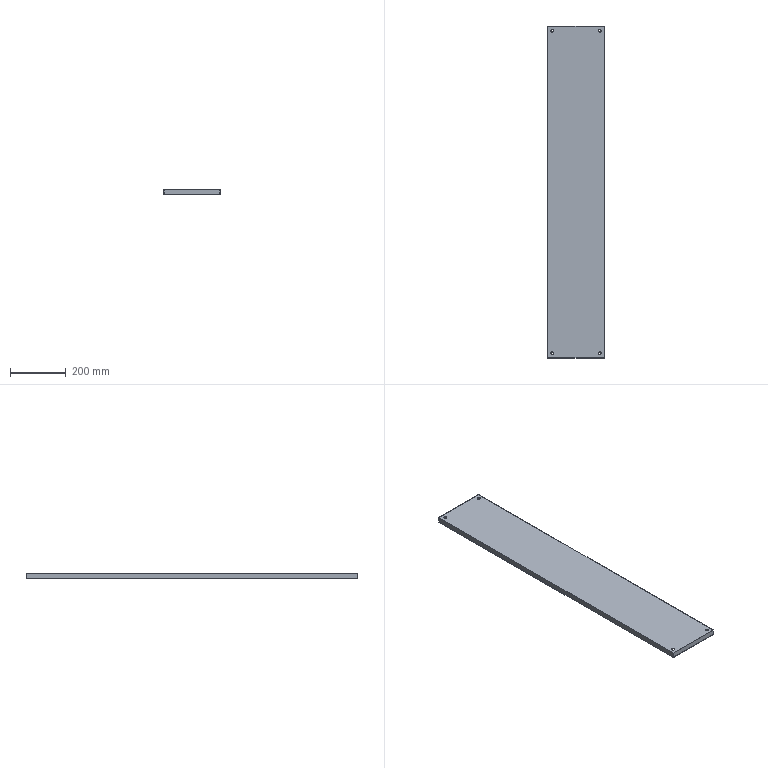Part | SolidWorks | features Extrusion 1, HoleWzd 1, ICE 1, Shell 1 | 1 solid | 32 faces | box 204 x 1196 x 20 mm | volume 684802 mm3 | cylinder 16 | plane 16 | commonest cylinder face diameters 6.6 x8 11 x8
STEP:
#1=CARTESIAN_POINT('',(-79.5,580.75,18.));
#2=VERTEX_POINT('',#1);
#3=CARTESIAN_POINT('',(-90.5,580.75,18.));
#4=VERTEX_POINT('',#3);
#5=CARTESIAN_POINT('',(-85.,580.75,18.));
#6=DIRECTION('',(0.,0.,-1.));
#7=DIRECTION('',(-1.,0.,0.));
#8=AXIS2_PLACEMENT_3D('',#5,#6,#7);
#9=CIRCLE('',#8,5.5);
#10=EDGE_CURVE('',#2,#4,#9,.T.);
#11=ORIENTED_EDGE('',*,*,#10,.T.);
#12=CARTESIAN_POINT('',(-90.5,580.75,20.));
#13=VERTEX_POINT('',#12);
#14=CARTESIAN_POINT('',(-90.5,580.75,20.));
#15=DIRECTION('',(0.,0.,1.));
#16=VECTOR('',#15,1000.);
#17=LINE('',#14,#16);
#18=EDGE_CURVE('',#4,#13,#17,.T.);
#19=ORIENTED_EDGE('',*,*,#18,.T.);
#20=CARTESIAN_POINT('',(-79.5,580.75,20.));
#21=VERTEX_POINT('',#20);
#22=CARTESIAN_POINT('',(-85.,580.75,20.));
#23=DIRECTION('',(0.,0.,1.));
#24=DIRECTION('',(1.,0.,0.));
#25=AXIS2_PLACEMENT_3D('',#22,#23,#24);
#26=CIRCLE('',#25,5.5);
#27=EDGE_CURVE('',#13,#21,#26,.T.);
#28=ORIENTED_EDGE('',*,*,#27,.T.);
#29=CARTESIAN_POINT('',(-79.5,580.75,20.));
#30=DIRECTION('',(0.,0.,1.));
#31=VECTOR('',#30,1000.);
#32=LINE('',#29,#31);
#33=EDGE_CURVE('',#2,#21,#32,.T.);
#34=ORIENTED_EDGE('',*,*,#33,.F.);
#35=EDGE_LOOP('',(#11,#19,#28,#34));
#36=FACE_OUTER_BOUND('',#35,.T.);
#37=CARTESIAN_POINT('',(-85.,580.75,20.));
#38=DIRECTION('',(0.,0.,1.));
#39=DIRECTION('',(1.,0.,0.));
#40=AXIS2_PLACEMENT_3D('',#37,#38,#39);
#41=CYLINDRICAL_SURFACE('',#40,5.5);
#42=ADVANCED_FACE('',(#36),#41,.F.);
#43=CARTESIAN_POINT('',(-88.3,580.75,0.));
#44=VERTEX_POINT('',#43);
#45=CARTESIAN_POINT('',(-81.7,580.75,0.));
#46=VERTEX_POINT('',#45);
#47=CARTESIAN_POINT('',(-85.,580.75,0.));
#48=DIRECTION('',(0.,0.,1.));
#49=DIRECTION('',(1.,0.,0.));
#50=AXIS2_PLACEMENT_3D('',#47,#48,#49);
#51=CIRCLE('',#50,3.3);
#52=EDGE_CURVE('',#44,#46,#51,.T.);
#53=ORIENTED_EDGE('',*,*,#52,.F.);
#54=CARTESIAN_POINT('',(-88.3,580.75,2.));
#55=VERTEX_POINT('',#54);
#56=CARTESIAN_POINT('',(-88.3,580.75,20.));
#57=DIRECTION('',(0.,0.,1.));
#58=VECTOR('',#57,1000.);
#59=LINE('',#56,#58);
#60=EDGE_CURVE('',#44,#55,#59,.T.);
#61=ORIENTED_EDGE('',*,*,#60,.T.);
#62=CARTESIAN_POINT('',(-81.7,580.75,2.));
#63=VERTEX_POINT('',#62);
#64=CARTESIAN_POINT('',(-85.,580.75,2.));
#65=DIRECTION('',(0.,0.,-1.));
#66=DIRECTION('',(-1.,0.,0.));
#67=AXIS2_PLACEMENT_3D('',#64,#65,#66);
#68=CIRCLE('',#67,3.3);
#69=EDGE_CURVE('',#63,#55,#68,.T.);
#70=ORIENTED_EDGE('',*,*,#69,.F.);
#71=CARTESIAN_POINT('',(-81.7,580.75,20.));
#72=DIRECTION('',(0.,0.,1.));
#73=VECTOR('',#72,1000.);
#74=LINE('',#71,#73);
#75=EDGE_CURVE('',#46,#63,#74,.T.);
#76=ORIENTED_EDGE('',*,*,#75,.F.);
#77=EDGE_LOOP('',(#53,#61,#70,#76));
#78=FACE_OUTER_BOUND('',#77,.T.);
#79=CARTESIAN_POINT('',(-85.,580.75,20.));
#80=DIRECTION('',(0.,0.,1.));
#81=DIRECTION('',(1.,0.,0.));
#82=AXIS2_PLACEMENT_3D('',#79,#80,#81);
#83=CYLINDRICAL_SURFACE('',#82,3.3);
#84=ADVANCED_FACE('',(#78),#83,.F.);
#85=CARTESIAN_POINT('',(-88.3,-580.75,0.));
#86=VERTEX_POINT('',#85);
#87=CARTESIAN_POINT('',(-81.7,-580.75,0.));
#88=VERTEX_POINT('',#87);
#89=CARTESIAN_POINT('',(-85.,-580.75,0.));
#90=DIRECTION('',(0.,0.,1.));
#91=DIRECTION('',(1.,0.,0.));
#92=AXIS2_PLACEMENT_3D('',#89,#90,#91);
#93=CIRCLE('',#92,3.3);
#94=EDGE_CURVE('',#86,#88,#93,.T.);
#95=ORIENTED_EDGE('',*,*,#94,.F.);
#96=CARTESIAN_POINT('',(-88.3,-580.75,2.));
#97=VERTEX_POINT('',#96);
#98=CARTESIAN_POINT('',(-88.3,-580.75,20.));
#99=DIRECTION('',(0.,0.,1.));
#100=VECTOR('',#99,1000.);
#101=LINE('',#98,#100);
#102=EDGE_CURVE('',#86,#97,#101,.T.);
#103=ORIENTED_EDGE('',*,*,#102,.T.);
#104=CARTESIAN_POINT('',(-81.7,-580.75,2.));
#105=VERTEX_POINT('',#104);
#106=CARTESIAN_POINT('',(-85.,-580.75,2.));
#107=DIRECTION('',(0.,0.,-1.));
#108=DIRECTION('',(-1.,0.,0.));
#109=AXIS2_PLACEMENT_3D('',#106,#107,#108);
#110=CIRCLE('',#109,3.3);
#111=EDGE_CURVE('',#105,#97,#110,.T.);
#112=ORIENTED_EDGE('',*,*,#111,.F.);
#113=CARTESIAN_POINT('',(-81.7,-580.75,20.));
#114=DIRECTION('',(0.,0.,1.));
#115=VECTOR('',#114,1000.);
#116=LINE('',#113,#115);
#117=EDGE_CURVE('',#88,#105,#116,.T.);
#118=ORIENTED_EDGE('',*,*,#117,.F.);
#119=EDGE_LOOP('',(#95,#103,#112,#118));
#120=FACE_OUTER_BOUND('',#119,.T.);
#121=CARTESIAN_POINT('',(-85.,-580.75,20.));
#122=DIRECTION('',(0.,0.,1.));
#123=DIRECTION('',(1.,0.,0.));
#124=AXIS2_PLACEMENT_3D('',#121,#122,#123);
#125=CYLINDRICAL_SURFACE('',#124,3.3);
#126=ADVANCED_FACE('',(#120),#125,.F.);
#127=CARTESIAN_POINT('',(-79.5,-580.75,18.));
#128=VERTEX_POINT('',#127);
#129=CARTESIAN_POINT('',(-90.5,-580.75,18.));
#130=VERTEX_POINT('',#129);
#131=CARTESIAN_POINT('',(-85.,-580.75,18.));
#132=DIRECTION('',(0.,0.,-1.));
#133=DIRECTION('',(-1.,0.,0.));
#134=AXIS2_PLACEMENT_3D('',#131,#132,#133);
#135=CIRCLE('',#134,5.5);
#136=EDGE_CURVE('',#128,#130,#135,.T.);
#137=ORIENTED_EDGE('',*,*,#136,.T.);
#138=CARTESIAN_POINT('',(-90.5,-580.75,20.));
#139=VERTEX_POINT('',#138);
#140=CARTESIAN_POINT('',(-90.5,-580.75,20.));
#141=DIRECTION('',(0.,0.,1.));
#142=VECTOR('',#141,1000.);
#143=LINE('',#140,#142);
#144=EDGE_CURVE('',#130,#139,#143,.T.);
#145=ORIENTED_EDGE('',*,*,#144,.T.);
#146=CARTESIAN_POINT('',(-79.5,-580.75,20.));
#147=VERTEX_POINT('',#146);
#148=CARTESIAN_POINT('',(-85.,-580.75,20.));
#149=DIRECTION('',(0.,0.,1.));
#150=DIRECTION('',(1.,0.,0.));
#151=AXIS2_PLACEMENT_3D('',#148,#149,#150);
#152=CIRCLE('',#151,5.5);
#153=EDGE_CURVE('',#139,#147,#152,.T.);
#154=ORIENTED_EDGE('',*,*,#153,.T.);
#155=CARTESIAN_POINT('',(-79.5,-580.75,20.));
#156=DIRECTION('',(0.,0.,1.));
#157=VECTOR('',#156,1000.);
#158=LINE('',#155,#157);
#159=EDGE_CURVE('',#128,#147,#158,.T.);
#160=ORIENTED_EDGE('',*,*,#159,.F.);
#161=EDGE_LOOP('',(#137,#145,#154,#160));
#162=FACE_OUTER_BOUND('',#161,.T.);
#163=CARTESIAN_POINT('',(-85.,-580.75,20.));
#164=DIRECTION('',(0.,0.,1.));
#165=DIRECTION('',(1.,0.,0.));
#166=AXIS2_PLACEMENT_3D('',#163,#164,#165);
#167=CYLINDRICAL_SURFACE('',#166,5.5);
#168=ADVANCED_FACE('',(#162),#167,.F.);
#169=CARTESIAN_POINT('',(90.5,-580.75,18.));
#170=VERTEX_POINT('',#169);
#171=CARTESIAN_POINT('',(79.5,-580.75,18.));
#172=VERTEX_POINT('',#171);
#173=CARTESIAN_POINT('',(85.,-580.75,18.));
#174=DIRECTION('',(0.,0.,-1.));
#175=DIRECTION('',(-1.,0.,0.));
#176=AXIS2_PLACEMENT_3D('',#173,#174,#175);
#177=CIRCLE('',#176,5.5);
#178=EDGE_CURVE('',#170,#172,#177,.T.);
#179=ORIENTED_EDGE('',*,*,#178,.T.);
#180=CARTESIAN_POINT('',(79.5,-580.75,20.));
#181=VERTEX_POINT('',#180);
#182=CARTESIAN_POINT('',(79.5,-580.75,20.));
#183=DIRECTION('',(0.,0.,1.));
#184=VECTOR('',#183,1000.);
#185=LINE('',#182,#184);
#186=EDGE_CURVE('',#172,#181,#185,.T.);
#187=ORIENTED_EDGE('',*,*,#186,.T.);
#188=CARTESIAN_POINT('',(90.5,-580.75,20.));
#189=VERTEX_POINT('',#188);
#190=CARTESIAN_POINT('',(85.,-580.75,20.));
#191=DIRECTION('',(0.,0.,1.));
#192=DIRECTION('',(1.,0.,0.));
#193=AXIS2_PLACEMENT_3D('',#190,#191,#192);
#194=CIRCLE('',#193,5.5);
#195=EDGE_CURVE('',#181,#189,#194,.T.);
#196=ORIENTED_EDGE('',*,*,#195,.T.);
#197=CARTESIAN_POINT('',(90.5,-580.75,20.));
#198=DIRECTION('',(0.,0.,1.));
#199=VECTOR('',#198,1000.);
#200=LINE('',#197,#199);
#201=EDGE_CURVE('',#170,#189,#200,.T.);
#202=ORIENTED_EDGE('',*,*,#201,.F.);
#203=EDGE_LOOP('',(#179,#187,#196,#202));
#204=FACE_OUTER_BOUND('',#203,.T.);
#205=CARTESIAN_POINT('',(85.,-580.75,20.));
#206=DIRECTION('',(0.,0.,1.));
#207=DIRECTION('',(1.,0.,0.));
#208=AXIS2_PLACEMENT_3D('',#205,#206,#207);
#209=CYLINDRICAL_SURFACE('',#208,5.5);
#210=ADVANCED_FACE('',(#204),#209,.F.);
#211=CARTESIAN_POINT('',(81.7,-580.75,0.));
#212=VERTEX_POINT('',#211);
#213=CARTESIAN_POINT('',(88.3,-580.75,0.));
#214=VERTEX_POINT('',#213);
#215=CARTESIAN_POINT('',(85.,-580.75,0.));
#216=DIRECTION('',(0.,0.,1.));
#217=DIRECTION('',(1.,0.,0.));
#218=AXIS2_PLACEMENT_3D('',#215,#216,#217);
#219=CIRCLE('',#218,3.3);
#220=EDGE_CURVE('',#212,#214,#219,.T.);
#221=ORIENTED_EDGE('',*,*,#220,.F.);
#222=CARTESIAN_POINT('',(81.7,-580.75,2.));
#223=VERTEX_POINT('',#222);
#224=CARTESIAN_POINT('',(81.7,-580.75,20.));
#225=DIRECTION('',(0.,0.,1.));
#226=VECTOR('',#225,1000.);
#227=LINE('',#224,#226);
#228=EDGE_CURVE('',#212,#223,#227,.T.);
#229=ORIENTED_EDGE('',*,*,#228,.T.);
#230=CARTESIAN_POINT('',(88.3,-580.75,2.));
#231=VERTEX_POINT('',#230);
#232=CARTESIAN_POINT('',(85.,-580.75,2.));
#233=DIRECTION('',(0.,0.,-1.));
#234=DIRECTION('',(-1.,0.,0.));
#235=AXIS2_PLACEMENT_3D('',#232,#233,#234);
#236=CIRCLE('',#235,3.3);
#237=EDGE_CURVE('',#231,#223,#236,.T.);
#238=ORIENTED_EDGE('',*,*,#237,.F.);
#239=CARTESIAN_POINT('',(88.3,-580.75,20.));
#240=DIRECTION('',(0.,0.,1.));
#241=VECTOR('',#240,1000.);
#242=LINE('',#239,#241);
#243=EDGE_CURVE('',#214,#231,#242,.T.);
#244=ORIENTED_EDGE('',*,*,#243,.F.);
#245=EDGE_LOOP('',(#221,#229,#238,#244));
#246=FACE_OUTER_BOUND('',#245,.T.);
#247=CARTESIAN_POINT('',(85.,-580.75,20.));
#248=DIRECTION('',(0.,0.,1.));
#249=DIRECTION('',(1.,0.,0.));
#250=AXIS2_PLACEMENT_3D('',#247,#248,#249);
#251=CYLINDRICAL_SURFACE('',#250,3.3);
#252=ADVANCED_FACE('',(#246),#251,.F.);
#253=CARTESIAN_POINT('',(81.7,580.75,0.));
#254=VERTEX_POINT('',#253);
#255=CARTESIAN_POINT('',(88.3,580.75,0.));
#256=VERTEX_POINT('',#255);
#257=CARTESIAN_POINT('',(85.,580.75,0.));
#258=DIRECTION('',(0.,0.,1.));
#259=DIRECTION('',(1.,0.,0.));
#260=AXIS2_PLACEMENT_3D('',#257,#258,#259);
#261=CIRCLE('',#260,3.3);
#262=EDGE_CURVE('',#254,#256,#261,.T.);
#263=ORIENTED_EDGE('',*,*,#262,.F.);
#264=CARTESIAN_POINT('',(81.7,580.75,2.));
#265=VERTEX_POINT('',#264);
#266=CARTESIAN_POINT('',(81.7,580.75,20.));
#267=DIRECTION('',(0.,0.,1.));
#268=VECTOR('',#267,1000.);
#269=LINE('',#266,#268);
#270=EDGE_CURVE('',#254,#265,#269,.T.);
#271=ORIENTED_EDGE('',*,*,#270,.T.);
#272=CARTESIAN_POINT('',(88.3,580.75,2.));
#273=VERTEX_POINT('',#272);
#274=CARTESIAN_POINT('',(85.,580.75,2.));
#275=DIRECTION('',(0.,0.,-1.));
#276=DIRECTION('',(-1.,0.,0.));
#277=AXIS2_PLACEMENT_3D('',#274,#275,#276);
#278=CIRCLE('',#277,3.3);
#279=EDGE_CURVE('',#273,#265,#278,.T.);
#280=ORIENTED_EDGE('',*,*,#279,.F.);
#281=CARTESIAN_POINT('',(88.3,580.75,20.));
#282=DIRECTION('',(0.,0.,1.));
#283=VECTOR('',#282,1000.);
#284=LINE('',#281,#283);
#285=EDGE_CURVE('',#256,#273,#284,.T.);
#286=ORIENTED_EDGE('',*,*,#285,.F.);
#287=EDGE_LOOP('',(#263,#271,#280,#286));
#288=FACE_OUTER_BOUND('',#287,.T.);
#289=CARTESIAN_POINT('',(85.,580.75,20.));
#290=DIRECTION('',(0.,0.,1.));
#291=DIRECTION('',(1.,0.,0.));
#292=AXIS2_PLACEMENT_3D('',#289,#290,#291);
#293=CYLINDRICAL_SURFACE('',#292,3.3);
#294=ADVANCED_FACE('',(#288),#293,.F.);
#295=CARTESIAN_POINT('',(90.5,580.75,18.));
#296=VERTEX_POINT('',#295);
#297=CARTESIAN_POINT('',(79.5,580.75,18.));
#298=VERTEX_POINT('',#297);
#299=CARTESIAN_POINT('',(85.,580.75,18.));
#300=DIRECTION('',(0.,0.,-1.));
#301=DIRECTION('',(-1.,0.,0.));
#302=AXIS2_PLACEMENT_3D('',#299,#300,#301);
#303=CIRCLE('',#302,5.5);
#304=EDGE_CURVE('',#296,#298,#303,.T.);
#305=ORIENTED_EDGE('',*,*,#304,.T.);
#306=CARTESIAN_POINT('',(79.5,580.75,20.));
#307=VERTEX_POINT('',#306);
#308=CARTESIAN_POINT('',(79.5,580.75,20.));
#309=DIRECTION('',(0.,0.,1.));
#310=VECTOR('',#309,1000.);
#311=LINE('',#308,#310);
#312=EDGE_CURVE('',#298,#307,#311,.T.);
#313=ORIENTED_EDGE('',*,*,#312,.T.);
#314=CARTESIAN_POINT('',(90.5,580.75,20.));
#315=VERTEX_POINT('',#314);
#316=CARTESIAN_POINT('',(85.,580.75,20.));
#317=DIRECTION('',(0.,0.,1.));
#318=DIRECTION('',(1.,0.,0.));
#319=AXIS2_PLACEMENT_3D('',#316,#317,#318);
#320=CIRCLE('',#319,5.5);
#321=EDGE_CURVE('',#307,#315,#320,.T.);
#322=ORIENTED_EDGE('',*,*,#321,.T.);
#323=CARTESIAN_POINT('',(90.5,580.75,20.));
#324=DIRECTION('',(0.,0.,1.));
#325=VECTOR('',#324,1000.);
#326=LINE('',#323,#325);
#327=EDGE_CURVE('',#296,#315,#326,.T.);
#328=ORIENTED_EDGE('',*,*,#327,.F.);
#329=EDGE_LOOP('',(#305,#313,#322,#328));
#330=FACE_OUTER_BOUND('',#329,.T.);
#331=CARTESIAN_POINT('',(85.,580.75,20.));
#332=DIRECTION('',(0.,0.,1.));
#333=DIRECTION('',(1.,0.,0.));
#334=AXIS2_PLACEMENT_3D('',#331,#332,#333);
#335=CYLINDRICAL_SURFACE('',#334,5.5);
#336=ADVANCED_FACE('',(#330),#335,.F.);
#337=CARTESIAN_POINT('',(85.,580.75,0.));
#338=DIRECTION('',(0.,0.,1.));
#339=DIRECTION('',(1.,0.,0.));
#340=AXIS2_PLACEMENT_3D('',#337,#338,#339);
#341=CIRCLE('',#340,3.3);
#342=EDGE_CURVE('',#256,#254,#341,.T.);
#343=ORIENTED_EDGE('',*,*,#342,.T.);
#344=ORIENTED_EDGE('',*,*,#262,.T.);
#345=EDGE_LOOP('',(#343,#344));
#346=FACE_BOUND('',#345,.T.);
#347=CARTESIAN_POINT('',(102.,-597.75,0.));
#348=VERTEX_POINT('',#347);
#349=CARTESIAN_POINT('',(102.,597.75,0.));
#350=VERTEX_POINT('',#349);
#351=CARTESIAN_POINT('',(102.,-597.75,0.));
#352=DIRECTION('',(0.,1.,0.));
#353=VECTOR('',#352,1000.);
#354=LINE('',#351,#353);
#355=EDGE_CURVE('',#348,#350,#354,.T.);
#356=ORIENTED_EDGE('',*,*,#355,.F.);
#357=CARTESIAN_POINT('',(-102.,-597.75,0.));
#358=VERTEX_POINT('',#357);
#359=CARTESIAN_POINT('',(-102.,-597.75,0.));
#360=DIRECTION('',(1.,0.,0.));
#361=VECTOR('',#360,1000.);
#362=LINE('',#359,#361);
#363=EDGE_CURVE('',#358,#348,#362,.T.);
#364=ORIENTED_EDGE('',*,*,#363,.F.);
#365=CARTESIAN_POINT('',(-102.,597.75,0.));
#366=VERTEX_POINT('',#365);
#367=CARTESIAN_POINT('',(-102.,-597.75,0.));
#368=DIRECTION('',(0.,-1.,0.));
#369=VECTOR('',#368,1000.);
#370=LINE('',#367,#369);
#371=EDGE_CURVE('',#366,#358,#370,.T.);
#372=ORIENTED_EDGE('',*,*,#371,.F.);
#373=CARTESIAN_POINT('',(-102.,597.75,0.));
#374=DIRECTION('',(-1.,0.,0.));
#375=VECTOR('',#374,1000.);
#376=LINE('',#373,#375);
#377=EDGE_CURVE('',#350,#366,#376,.T.);
#378=ORIENTED_EDGE('',*,*,#377,.F.);
#379=EDGE_LOOP('',(#356,#364,#372,#378));
#380=FACE_OUTER_BOUND('',#379,.T.);
#381=CARTESIAN_POINT('',(82.,-577.75,0.));
#382=VERTEX_POINT('',#381);
#383=CARTESIAN_POINT('',(-82.,-577.75,0.));
#384=VERTEX_POINT('',#383);
#385=CARTESIAN_POINT('',(82.,-577.75,0.));
#386=DIRECTION('',(-1.,0.,0.));
#387=VECTOR('',#386,1000.);
#388=LINE('',#385,#387);
#389=EDGE_CURVE('',#382,#384,#388,.T.);
#390=ORIENTED_EDGE('',*,*,#389,.F.);
#391=CARTESIAN_POINT('',(82.,577.75,0.));
#392=VERTEX_POINT('',#391);
#393=CARTESIAN_POINT('',(82.,-577.75,0.));
#394=DIRECTION('',(0.,1.,0.));
#395=VECTOR('',#394,1000.);
#396=LINE('',#393,#395);
#397=EDGE_CURVE('',#382,#392,#396,.T.);
#398=ORIENTED_EDGE('',*,*,#397,.T.);
#399=CARTESIAN_POINT('',(-82.,577.75,0.));
#400=VERTEX_POINT('',#399);
#401=CARTESIAN_POINT('',(82.,577.75,0.));
#402=DIRECTION('',(-1.,0.,0.));
#403=VECTOR('',#402,1000.);
#404=LINE('',#401,#403);
#405=EDGE_CURVE('',#392,#400,#404,.T.);
#406=ORIENTED_EDGE('',*,*,#405,.T.);
#407=CARTESIAN_POINT('',(-82.,-577.75,0.));
#408=DIRECTION('',(0.,1.,0.));
#409=VECTOR('',#408,1000.);
#410=LINE('',#407,#409);
#411=EDGE_CURVE('',#384,#400,#410,.T.);
#412=ORIENTED_EDGE('',*,*,#411,.F.);
#413=EDGE_LOOP('',(#390,#398,#406,#412));
#414=FACE_BOUND('',#413,.T.);
#415=CARTESIAN_POINT('',(85.,-580.75,0.));
#416=DIRECTION('',(0.,0.,1.));
#417=DIRECTION('',(1.,0.,0.));
#418=AXIS2_PLACEMENT_3D('',#415,#416,#417);
#419=CIRCLE('',#418,3.3);
#420=EDGE_CURVE('',#214,#212,#419,.T.);
#421=ORIENTED_EDGE('',*,*,#420,.T.);
#422=ORIENTED_EDGE('',*,*,#220,.T.);
#423=EDGE_LOOP('',(#421,#422));
#424=FACE_BOUND('',#423,.T.);
#425=CARTESIAN_POINT('',(-85.,-580.75,0.));
#426=DIRECTION('',(0.,0.,1.));
#427=DIRECTION('',(1.,0.,0.));
#428=AXIS2_PLACEMENT_3D('',#425,#426,#427);
#429=CIRCLE('',#428,3.3);
#430=EDGE_CURVE('',#88,#86,#429,.T.);
#431=ORIENTED_EDGE('',*,*,#430,.T.);
#432=ORIENTED_EDGE('',*,*,#94,.T.);
#433=EDGE_LOOP('',(#431,#432));
#434=FACE_BOUND('',#433,.T.);
#435=CARTESIAN_POINT('',(-85.,580.75,0.));
#436=DIRECTION('',(0.,0.,1.));
#437=DIRECTION('',(1.,0.,0.));
#438=AXIS2_PLACEMENT_3D('',#435,#436,#437);
#439=CIRCLE('',#438,3.3);
#440=EDGE_CURVE('',#46,#44,#439,.T.);
#441=ORIENTED_EDGE('',*,*,#440,.T.);
#442=ORIENTED_EDGE('',*,*,#52,.T.);
#443=EDGE_LOOP('',(#441,#442));
#444=FACE_BOUND('',#443,.T.);
#445=CARTESIAN_POINT('',(0.,0.,0.));
#446=DIRECTION('',(0.,0.,-1.));
#447=DIRECTION('',(-1.,0.,0.));
#448=AXIS2_PLACEMENT_3D('',#445,#446,#447);
#449=PLANE('',#448);
#450=ADVANCED_FACE('',(#346,#380,#414,#424,#434,#444),#449,.T.);
#451=ORIENTED_EDGE('',*,*,#355,.T.);
#452=CARTESIAN_POINT('',(102.,597.75,20.));
#453=VERTEX_POINT('',#452);
#454=CARTESIAN_POINT('',(102.,597.75,20.));
#455=DIRECTION('',(0.,0.,-1.));
#456=VECTOR('',#455,1000.);
#457=LINE('',#454,#456);
#458=EDGE_CURVE('',#453,#350,#457,.T.);
#459=ORIENTED_EDGE('',*,*,#458,.F.);
#460=CARTESIAN_POINT('',(102.,-597.75,20.));
#461=VERTEX_POINT('',#460);
#462=CARTESIAN_POINT('',(102.,-597.75,20.));
#463=DIRECTION('',(0.,1.,0.));
#464=VECTOR('',#463,1000.);
#465=LINE('',#462,#464);
#466=EDGE_CURVE('',#461,#453,#465,.T.);
#467=ORIENTED_EDGE('',*,*,#466,.F.);
#468=CARTESIAN_POINT('',(102.,-597.75,20.));
#469=DIRECTION('',(0.,0.,-1.));
#470=VECTOR('',#469,1000.);
#471=LINE('',#468,#470);
#472=EDGE_CURVE('',#461,#348,#471,.T.);
#473=ORIENTED_EDGE('',*,*,#472,.T.);
#474=EDGE_LOOP('',(#451,#459,#467,#473));
#475=FACE_OUTER_BOUND('',#474,.T.);
#476=CARTESIAN_POINT('',(102.,-597.75,20.));
#477=DIRECTION('',(-1.,0.,0.));
#478=DIRECTION('',(0.,0.,1.));
#479=AXIS2_PLACEMENT_3D('',#476,#477,#478);
#480=PLANE('',#479);
#481=ADVANCED_FACE('',(#475),#480,.F.);
#482=ORIENTED_EDGE('',*,*,#377,.T.);
#483=CARTESIAN_POINT('',(-102.,597.75,20.));
#484=VERTEX_POINT('',#483);
#485=CARTESIAN_POINT('',(-102.,597.75,20.));
#486=DIRECTION('',(0.,0.,-1.));
#487=VECTOR('',#486,1000.);
#488=LINE('',#485,#487);
#489=EDGE_CURVE('',#484,#366,#488,.T.);
#490=ORIENTED_EDGE('',*,*,#489,.F.);
#491=CARTESIAN_POINT('',(-102.,597.75,20.));
#492=DIRECTION('',(-1.,0.,0.));
#493=VECTOR('',#492,1000.);
#494=LINE('',#491,#493);
#495=EDGE_CURVE('',#453,#484,#494,.T.);
#496=ORIENTED_EDGE('',*,*,#495,.F.);
#497=ORIENTED_EDGE('',*,*,#458,.T.);
#498=EDGE_LOOP('',(#482,#490,#496,#497));
#499=FACE_OUTER_BOUND('',#498,.T.);
#500=CARTESIAN_POINT('',(-102.,597.75,20.));
#501=DIRECTION('',(0.,-1.,0.));
#502=DIRECTION('',(0.,0.,-1.));
#503=AXIS2_PLACEMENT_3D('',#500,#501,#502);
#504=PLANE('',#503);
#505=ADVANCED_FACE('',(#499),#504,.F.);
#506=ORIENTED_EDGE('',*,*,#371,.T.);
#507=CARTESIAN_POINT('',(-102.,-597.75,20.));
#508=VERTEX_POINT('',#507);
#509=CARTESIAN_POINT('',(-102.,-597.75,20.));
#510=DIRECTION('',(0.,0.,-1.));
#511=VECTOR('',#510,1000.);
#512=LINE('',#509,#511);
#513=EDGE_CURVE('',#508,#358,#512,.T.);
#514=ORIENTED_EDGE('',*,*,#513,.F.);
#515=CARTESIAN_POINT('',(-102.,-597.75,20.));
#516=DIRECTION('',(0.,-1.,0.));
#517=VECTOR('',#516,1000.);
#518=LINE('',#515,#517);
#519=EDGE_CURVE('',#484,#508,#518,.T.);
#520=ORIENTED_EDGE('',*,*,#519,.F.);
#521=ORIENTED_EDGE('',*,*,#489,.T.);
#522=EDGE_LOOP('',(#506,#514,#520,#521));
#523=FACE_OUTER_BOUND('',#522,.T.);
#524=CARTESIAN_POINT('',(-102.,-597.75,20.));
#525=DIRECTION('',(1.,0.,0.));
#526=DIRECTION('',(0.,0.,-1.));
#527=AXIS2_PLACEMENT_3D('',#524,#525,#526);
#528=PLANE('',#527);
#529=ADVANCED_FACE('',(#523),#528,.F.);
#530=ORIENTED_EDGE('',*,*,#363,.T.);
#531=ORIENTED_EDGE('',*,*,#472,.F.);
#532=CARTESIAN_POINT('',(-102.,-597.75,20.));
#533=DIRECTION('',(1.,0.,0.));
#534=VECTOR('',#533,1000.);
#535=LINE('',#532,#534);
#536=EDGE_CURVE('',#508,#461,#535,.T.);
#537=ORIENTED_EDGE('',*,*,#536,.F.);
#538=ORIENTED_EDGE('',*,*,#513,.T.);
#539=EDGE_LOOP('',(#530,#531,#537,#538));
#540=FACE_OUTER_BOUND('',#539,.T.);
#541=CARTESIAN_POINT('',(-102.,-597.75,20.));
#542=DIRECTION('',(0.,1.,0.));
#543=DIRECTION('',(0.,0.,1.));
#544=AXIS2_PLACEMENT_3D('',#541,#542,#543);
#545=PLANE('',#544);
#546=ADVANCED_FACE('',(#540),#545,.F.);
#547=CARTESIAN_POINT('',(-85.,580.75,20.));
#548=DIRECTION('',(0.,0.,1.));
#549=DIRECTION('',(1.,0.,0.));
#550=AXIS2_PLACEMENT_3D('',#547,#548,#549);
#551=CIRCLE('',#550,5.5);
#552=EDGE_CURVE('',#21,#13,#551,.T.);
#553=ORIENTED_EDGE('',*,*,#552,.F.);
#554=ORIENTED_EDGE('',*,*,#27,.F.);
#555=EDGE_LOOP('',(#553,#554));
#556=FACE_BOUND('',#555,.T.);
#557=CARTESIAN_POINT('',(-85.,-580.75,20.));
#558=DIRECTION('',(0.,0.,1.));
#559=DIRECTION('',(1.,0.,0.));
#560=AXIS2_PLACEMENT_3D('',#557,#558,#559);
#561=CIRCLE('',#560,5.5);
#562=EDGE_CURVE('',#147,#139,#561,.T.);
#563=ORIENTED_EDGE('',*,*,#562,.F.);
#564=ORIENTED_EDGE('',*,*,#153,.F.);
#565=EDGE_LOOP('',(#563,#564));
#566=FACE_BOUND('',#565,.T.);
#567=CARTESIAN_POINT('',(85.,-580.75,20.));
#568=DIRECTION('',(0.,0.,1.));
#569=DIRECTION('',(1.,0.,0.));
#570=AXIS2_PLACEMENT_3D('',#567,#568,#569);
#571=CIRCLE('',#570,5.5);
#572=EDGE_CURVE('',#189,#181,#571,.T.);
#573=ORIENTED_EDGE('',*,*,#572,.F.);
#574=ORIENTED_EDGE('',*,*,#195,.F.);
#575=EDGE_LOOP('',(#573,#574));
#576=FACE_BOUND('',#575,.T.);
#577=CARTESIAN_POINT('',(85.,580.75,20.));
#578=DIRECTION('',(0.,0.,1.));
#579=DIRECTION('',(1.,0.,0.));
#580=AXIS2_PLACEMENT_3D('',#577,#578,#579);
#581=CIRCLE('',#580,5.5);
#582=EDGE_CURVE('',#315,#307,#581,.T.);
#583=ORIENTED_EDGE('',*,*,#582,.F.);
#584=ORIENTED_EDGE('',*,*,#321,.F.);
#585=EDGE_LOOP('',(#583,#584));
#586=FACE_BOUND('',#585,.T.);
#587=ORIENTED_EDGE('',*,*,#466,.T.);
#588=ORIENTED_EDGE('',*,*,#495,.T.);
#589=ORIENTED_EDGE('',*,*,#519,.T.);
#590=ORIENTED_EDGE('',*,*,#536,.T.);
#591=EDGE_LOOP('',(#587,#588,#589,#590));
#592=FACE_OUTER_BOUND('',#591,.T.);
#593=CARTESIAN_POINT('',(0.,0.,20.));
#594=DIRECTION('',(0.,0.,-1.));
#595=DIRECTION('',(-1.,0.,0.));
#596=AXIS2_PLACEMENT_3D('',#593,#594,#595);
#597=PLANE('',#596);
#598=ADVANCED_FACE('',(#556,#566,#576,#586,#592),#597,.F.);
#599=ORIENTED_EDGE('',*,*,#397,.F.);
#600=CARTESIAN_POINT('',(82.,-577.75,2.));
#601=VERTEX_POINT('',#600);
#602=CARTESIAN_POINT('',(82.,-577.75,2.));
#603=DIRECTION('',(0.,0.,-1.));
#604=VECTOR('',#603,1000.);
#605=LINE('',#602,#604);
#606=EDGE_CURVE('',#601,#382,#605,.T.);
#607=ORIENTED_EDGE('',*,*,#606,.F.);
#608=CARTESIAN_POINT('',(82.,577.75,2.));
#609=VERTEX_POINT('',#608);
#610=CARTESIAN_POINT('',(82.,-577.75,2.));
#611=DIRECTION('',(0.,1.,0.));
#612=VECTOR('',#611,1000.);
#613=LINE('',#610,#612);
#614=EDGE_CURVE('',#601,#609,#613,.T.);
#615=ORIENTED_EDGE('',*,*,#614,.T.);
#616=CARTESIAN_POINT('',(82.,577.75,2.));
#617=DIRECTION('',(0.,0.,-1.));
#618=VECTOR('',#617,1000.);
#619=LINE('',#616,#618);
#620=EDGE_CURVE('',#609,#392,#619,.T.);
#621=ORIENTED_EDGE('',*,*,#620,.T.);
#622=EDGE_LOOP('',(#599,#607,#615,#621));
#623=FACE_OUTER_BOUND('',#622,.T.);
#624=CARTESIAN_POINT('',(82.,-577.75,2.));
#625=DIRECTION('',(-1.,0.,0.));
#626=DIRECTION('',(0.,0.,1.));
#627=AXIS2_PLACEMENT_3D('',#624,#625,#626);
#628=PLANE('',#627);
#629=ADVANCED_FACE('',(#623),#628,.T.);
#630=ORIENTED_EDGE('',*,*,#405,.F.);
#631=ORIENTED_EDGE('',*,*,#620,.F.);
#632=CARTESIAN_POINT('',(-82.,577.75,2.));
#633=VERTEX_POINT('',#632);
#634=CARTESIAN_POINT('',(82.,577.75,2.));
#635=DIRECTION('',(-1.,0.,0.));
#636=VECTOR('',#635,1000.);
#637=LINE('',#634,#636);
#638=EDGE_CURVE('',#609,#633,#637,.T.);
#639=ORIENTED_EDGE('',*,*,#638,.T.);
#640=CARTESIAN_POINT('',(-82.,577.75,2.));
#641=DIRECTION('',(0.,0.,-1.));
#642=VECTOR('',#641,1000.);
#643=LINE('',#640,#642);
#644=EDGE_CURVE('',#633,#400,#643,.T.);
#645=ORIENTED_EDGE('',*,*,#644,.T.);
#646=EDGE_LOOP('',(#630,#631,#639,#645));
#647=FACE_OUTER_BOUND('',#646,.T.);
#648=CARTESIAN_POINT('',(82.,577.75,2.));
#649=DIRECTION('',(0.,-1.,0.));
#650=DIRECTION('',(0.,0.,-1.));
#651=AXIS2_PLACEMENT_3D('',#648,#649,#650);
#652=PLANE('',#651);
#653=ADVANCED_FACE('',(#647),#652,.T.);
#654=ORIENTED_EDGE('',*,*,#411,.T.);
#655=ORIENTED_EDGE('',*,*,#644,.F.);
#656=CARTESIAN_POINT('',(-82.,-577.75,2.));
#657=VERTEX_POINT('',#656);
#658=CARTESIAN_POINT('',(-82.,-577.75,2.));
#659=DIRECTION('',(0.,1.,0.));
#660=VECTOR('',#659,1000.);
#661=LINE('',#658,#660);
#662=EDGE_CURVE('',#657,#633,#661,.T.);
#663=ORIENTED_EDGE('',*,*,#662,.F.);
#664=CARTESIAN_POINT('',(-82.,-577.75,2.));
#665=DIRECTION('',(0.,0.,-1.));
#666=VECTOR('',#665,1000.);
#667=LINE('',#664,#666);
#668=EDGE_CURVE('',#657,#384,#667,.T.);
#669=ORIENTED_EDGE('',*,*,#668,.T.);
#670=EDGE_LOOP('',(#654,#655,#663,#669));
#671=FACE_OUTER_BOUND('',#670,.T.);
#672=CARTESIAN_POINT('',(-82.,-577.75,2.));
#673=DIRECTION('',(-1.,0.,0.));
#674=DIRECTION('',(0.,0.,1.));
#675=AXIS2_PLACEMENT_3D('',#672,#673,#674);
#676=PLANE('',#675);
#677=ADVANCED_FACE('',(#671),#676,.F.);
#678=ORIENTED_EDGE('',*,*,#389,.T.);
#679=ORIENTED_EDGE('',*,*,#668,.F.);
#680=CARTESIAN_POINT('',(82.,-577.75,2.));
#681=DIRECTION('',(-1.,0.,0.));
#682=VECTOR('',#681,1000.);
#683=LINE('',#680,#682);
#684=EDGE_CURVE('',#601,#657,#683,.T.);
#685=ORIENTED_EDGE('',*,*,#684,.F.);
#686=ORIENTED_EDGE('',*,*,#606,.T.);
#687=EDGE_LOOP('',(#678,#679,#685,#686));
#688=FACE_OUTER_BOUND('',#687,.T.);
#689=CARTESIAN_POINT('',(82.,-577.75,2.));
#690=DIRECTION('',(0.,-1.,0.));
#691=DIRECTION('',(0.,0.,-1.));
#692=AXIS2_PLACEMENT_3D('',#689,#690,#691);
#693=PLANE('',#692);
#694=ADVANCED_FACE('',(#688),#693,.F.);
#695=ORIENTED_EDGE('',*,*,#69,.T.);
#696=CARTESIAN_POINT('',(-85.,580.75,2.));
#697=DIRECTION('',(0.,0.,-1.));
#698=DIRECTION('',(-1.,0.,0.));
#699=AXIS2_PLACEMENT_3D('',#696,#697,#698);
#700=CIRCLE('',#699,3.3);
#701=EDGE_CURVE('',#55,#63,#700,.T.);
#702=ORIENTED_EDGE('',*,*,#701,.T.);
#703=EDGE_LOOP('',(#695,#702));
#704=FACE_BOUND('',#703,.T.);
#705=ORIENTED_EDGE('',*,*,#111,.T.);
#706=CARTESIAN_POINT('',(-85.,-580.75,2.));
#707=DIRECTION('',(0.,0.,-1.));
#708=DIRECTION('',(-1.,0.,0.));
#709=AXIS2_PLACEMENT_3D('',#706,#707,#708);
#710=CIRCLE('',#709,3.3);
#711=EDGE_CURVE('',#97,#105,#710,.T.);
#712=ORIENTED_EDGE('',*,*,#711,.T.);
#713=EDGE_LOOP('',(#705,#712));
#714=FACE_BOUND('',#713,.T.);
#715=ORIENTED_EDGE('',*,*,#237,.T.);
#716=CARTESIAN_POINT('',(85.,-580.75,2.));
#717=DIRECTION('',(0.,0.,-1.));
#718=DIRECTION('',(-1.,0.,0.));
#719=AXIS2_PLACEMENT_3D('',#716,#717,#718);
#720=CIRCLE('',#719,3.3);
#721=EDGE_CURVE('',#223,#231,#720,.T.);
#722=ORIENTED_EDGE('',*,*,#721,.T.);
#723=EDGE_LOOP('',(#715,#722));
#724=FACE_BOUND('',#723,.T.);
#725=ORIENTED_EDGE('',*,*,#279,.T.);
#726=CARTESIAN_POINT('',(85.,580.75,2.));
#727=DIRECTION('',(0.,0.,-1.));
#728=DIRECTION('',(-1.,0.,0.));
#729=AXIS2_PLACEMENT_3D('',#726,#727,#728);
#730=CIRCLE('',#729,3.3);
#731=EDGE_CURVE('',#265,#273,#730,.T.);
#732=ORIENTED_EDGE('',*,*,#731,.T.);
#733=EDGE_LOOP('',(#725,#732));
#734=FACE_BOUND('',#733,.T.);
#735=CARTESIAN_POINT('',(100.,-595.75,2.));
#736=VERTEX_POINT('',#735);
#737=CARTESIAN_POINT('',(100.,595.75,2.));
#738=VERTEX_POINT('',#737);
#739=CARTESIAN_POINT('',(100.,0.,2.));
#740=DIRECTION('',(0.,1.,0.));
#741=VECTOR('',#740,1000.);
#742=LINE('',#739,#741);
#743=EDGE_CURVE('',#736,#738,#742,.T.);
#744=ORIENTED_EDGE('',*,*,#743,.T.);
#745=CARTESIAN_POINT('',(-100.,595.75,2.));
#746=VERTEX_POINT('',#745);
#747=CARTESIAN_POINT('',(0.,595.75,2.));
#748=DIRECTION('',(-1.,0.,0.));
#749=VECTOR('',#748,1000.);
#750=LINE('',#747,#749);
#751=EDGE_CURVE('',#738,#746,#750,.T.);
#752=ORIENTED_EDGE('',*,*,#751,.T.);
#753=CARTESIAN_POINT('',(-100.,-595.75,2.));
#754=VERTEX_POINT('',#753);
#755=CARTESIAN_POINT('',(-100.,0.,2.));
#756=DIRECTION('',(0.,-1.,0.));
#757=VECTOR('',#756,1000.);
#758=LINE('',#755,#757);
#759=EDGE_CURVE('',#746,#754,#758,.T.);
#760=ORIENTED_EDGE('',*,*,#759,.T.);
#761=CARTESIAN_POINT('',(0.,-595.75,2.));
#762=DIRECTION('',(1.,0.,0.));
#763=VECTOR('',#762,1000.);
#764=LINE('',#761,#763);
#765=EDGE_CURVE('',#754,#736,#764,.T.);
#766=ORIENTED_EDGE('',*,*,#765,.T.);
#767=EDGE_LOOP('',(#744,#752,#760,#766));
#768=FACE_OUTER_BOUND('',#767,.T.);
#769=ORIENTED_EDGE('',*,*,#684,.T.);
#770=ORIENTED_EDGE('',*,*,#662,.T.);
#771=ORIENTED_EDGE('',*,*,#638,.F.);
#772=ORIENTED_EDGE('',*,*,#614,.F.);
#773=EDGE_LOOP('',(#769,#770,#771,#772));
#774=FACE_BOUND('',#773,.T.);
#775=CARTESIAN_POINT('',(0.,0.,2.));
#776=DIRECTION('',(0.,0.,-1.));
#777=DIRECTION('',(-1.,0.,0.));
#778=AXIS2_PLACEMENT_3D('',#775,#776,#777);
#779=PLANE('',#778);
#780=ADVANCED_FACE('',(#704,#714,#724,#734,#768,#774),#779,.F.);
#781=ORIENTED_EDGE('',*,*,#743,.F.);
#782=CARTESIAN_POINT('',(100.,-595.75,18.));
#783=VERTEX_POINT('',#782);
#784=CARTESIAN_POINT('',(100.,-595.75,20.));
#785=DIRECTION('',(0.,0.,-1.));
#786=VECTOR('',#785,1000.);
#787=LINE('',#784,#786);
#788=EDGE_CURVE('',#783,#736,#787,.T.);
#789=ORIENTED_EDGE('',*,*,#788,.F.);
#790=CARTESIAN_POINT('',(100.,595.75,18.));
#791=VERTEX_POINT('',#790);
#792=CARTESIAN_POINT('',(100.,0.,18.));
#793=DIRECTION('',(0.,1.,0.));
#794=VECTOR('',#793,1000.);
#795=LINE('',#792,#794);
#796=EDGE_CURVE('',#783,#791,#795,.T.);
#797=ORIENTED_EDGE('',*,*,#796,.T.);
#798=CARTESIAN_POINT('',(100.,595.75,20.));
#799=DIRECTION('',(0.,0.,-1.));
#800=VECTOR('',#799,1000.);
#801=LINE('',#798,#800);
#802=EDGE_CURVE('',#791,#738,#801,.T.);
#803=ORIENTED_EDGE('',*,*,#802,.T.);
#804=EDGE_LOOP('',(#781,#789,#797,#803));
#805=FACE_OUTER_BOUND('',#804,.T.);
#806=CARTESIAN_POINT('',(100.,-597.75,20.));
#807=DIRECTION('',(-1.,0.,0.));
#808=DIRECTION('',(0.,0.,1.));
#809=AXIS2_PLACEMENT_3D('',#806,#807,#808);
#810=PLANE('',#809);
#811=ADVANCED_FACE('',(#805),#810,.T.);
#812=ORIENTED_EDGE('',*,*,#751,.F.);
#813=ORIENTED_EDGE('',*,*,#802,.F.);
#814=CARTESIAN_POINT('',(-100.,595.75,18.));
#815=VERTEX_POINT('',#814);
#816=CARTESIAN_POINT('',(0.,595.75,18.));
#817=DIRECTION('',(-1.,0.,0.));
#818=VECTOR('',#817,1000.);
#819=LINE('',#816,#818);
#820=EDGE_CURVE('',#791,#815,#819,.T.);
#821=ORIENTED_EDGE('',*,*,#820,.T.);
#822=CARTESIAN_POINT('',(-100.,595.75,20.));
#823=DIRECTION('',(0.,0.,-1.));
#824=VECTOR('',#823,1000.);
#825=LINE('',#822,#824);
#826=EDGE_CURVE('',#815,#746,#825,.T.);
#827=ORIENTED_EDGE('',*,*,#826,.T.);
#828=EDGE_LOOP('',(#812,#813,#821,#827));
#829=FACE_OUTER_BOUND('',#828,.T.);
#830=CARTESIAN_POINT('',(-102.,595.75,20.));
#831=DIRECTION('',(0.,-1.,0.));
#832=DIRECTION('',(0.,0.,-1.));
#833=AXIS2_PLACEMENT_3D('',#830,#831,#832);
#834=PLANE('',#833);
#835=ADVANCED_FACE('',(#829),#834,.T.);
#836=ORIENTED_EDGE('',*,*,#759,.F.);
#837=ORIENTED_EDGE('',*,*,#826,.F.);
#838=CARTESIAN_POINT('',(-100.,-595.75,18.));
#839=VERTEX_POINT('',#838);
#840=CARTESIAN_POINT('',(-100.,0.,18.));
#841=DIRECTION('',(0.,-1.,0.));
#842=VECTOR('',#841,1000.);
#843=LINE('',#840,#842);
#844=EDGE_CURVE('',#815,#839,#843,.T.);
#845=ORIENTED_EDGE('',*,*,#844,.T.);
#846=CARTESIAN_POINT('',(-100.,-595.75,20.));
#847=DIRECTION('',(0.,0.,-1.));
#848=VECTOR('',#847,1000.);
#849=LINE('',#846,#848);
#850=EDGE_CURVE('',#839,#754,#849,.T.);
#851=ORIENTED_EDGE('',*,*,#850,.T.);
#852=EDGE_LOOP('',(#836,#837,#845,#851));
#853=FACE_OUTER_BOUND('',#852,.T.);
#854=CARTESIAN_POINT('',(-100.,-597.75,20.));
#855=DIRECTION('',(1.,0.,0.));
#856=DIRECTION('',(0.,0.,-1.));
#857=AXIS2_PLACEMENT_3D('',#854,#855,#856);
#858=PLANE('',#857);
#859=ADVANCED_FACE('',(#853),#858,.T.);
#860=ORIENTED_EDGE('',*,*,#765,.F.);
#861=ORIENTED_EDGE('',*,*,#850,.F.);
#862=CARTESIAN_POINT('',(0.,-595.75,18.));
#863=DIRECTION('',(1.,0.,0.));
#864=VECTOR('',#863,1000.);
#865=LINE('',#862,#864);
#866=EDGE_CURVE('',#839,#783,#865,.T.);
#867=ORIENTED_EDGE('',*,*,#866,.T.);
#868=ORIENTED_EDGE('',*,*,#788,.T.);
#869=EDGE_LOOP('',(#860,#861,#867,#868));
#870=FACE_OUTER_BOUND('',#869,.T.);
#871=CARTESIAN_POINT('',(-102.,-595.75,20.));
#872=DIRECTION('',(0.,1.,0.));
#873=DIRECTION('',(0.,0.,1.));
#874=AXIS2_PLACEMENT_3D('',#871,#872,#873);
#875=PLANE('',#874);
#876=ADVANCED_FACE('',(#870),#875,.T.);
#877=ORIENTED_EDGE('',*,*,#10,.F.);
#878=CARTESIAN_POINT('',(-85.,580.75,18.));
#879=DIRECTION('',(0.,0.,-1.));
#880=DIRECTION('',(-1.,0.,0.));
#881=AXIS2_PLACEMENT_3D('',#878,#879,#880);
#882=CIRCLE('',#881,5.5);
#883=EDGE_CURVE('',#4,#2,#882,.T.);
#884=ORIENTED_EDGE('',*,*,#883,.F.);
#885=EDGE_LOOP('',(#877,#884));
#886=FACE_BOUND('',#885,.T.);
#887=ORIENTED_EDGE('',*,*,#136,.F.);
#888=CARTESIAN_POINT('',(-85.,-580.75,18.));
#889=DIRECTION('',(0.,0.,-1.));
#890=DIRECTION('',(-1.,0.,0.));
#891=AXIS2_PLACEMENT_3D('',#888,#889,#890);
#892=CIRCLE('',#891,5.5);
#893=EDGE_CURVE('',#130,#128,#892,.T.);
#894=ORIENTED_EDGE('',*,*,#893,.F.);
#895=EDGE_LOOP('',(#887,#894));
#896=FACE_BOUND('',#895,.T.);
#897=ORIENTED_EDGE('',*,*,#178,.F.);
#898=CARTESIAN_POINT('',(85.,-580.75,18.));
#899=DIRECTION('',(0.,0.,-1.));
#900=DIRECTION('',(-1.,0.,0.));
#901=AXIS2_PLACEMENT_3D('',#898,#899,#900);
#902=CIRCLE('',#901,5.5);
#903=EDGE_CURVE('',#172,#170,#902,.T.);
#904=ORIENTED_EDGE('',*,*,#903,.F.);
#905=EDGE_LOOP('',(#897,#904));
#906=FACE_BOUND('',#905,.T.);
#907=ORIENTED_EDGE('',*,*,#304,.F.);
#908=CARTESIAN_POINT('',(85.,580.75,18.));
#909=DIRECTION('',(0.,0.,-1.));
#910=DIRECTION('',(-1.,0.,0.));
#911=AXIS2_PLACEMENT_3D('',#908,#909,#910);
#912=CIRCLE('',#911,5.5);
#913=EDGE_CURVE('',#298,#296,#912,.T.);
#914=ORIENTED_EDGE('',*,*,#913,.F.);
#915=EDGE_LOOP('',(#907,#914));
#916=FACE_BOUND('',#915,.T.);
#917=ORIENTED_EDGE('',*,*,#796,.F.);
#918=ORIENTED_EDGE('',*,*,#866,.F.);
#919=ORIENTED_EDGE('',*,*,#844,.F.);
#920=ORIENTED_EDGE('',*,*,#820,.F.);
#921=EDGE_LOOP('',(#917,#918,#919,#920));
#922=FACE_OUTER_BOUND('',#921,.T.);
#923=CARTESIAN_POINT('',(0.,0.,18.));
#924=DIRECTION('',(0.,0.,-1.));
#925=DIRECTION('',(-1.,0.,0.));
#926=AXIS2_PLACEMENT_3D('',#923,#924,#925);
#927=PLANE('',#926);
#928=ADVANCED_FACE('',(#886,#896,#906,#916,#922),#927,.T.);
#929=ORIENTED_EDGE('',*,*,#312,.F.);
#930=ORIENTED_EDGE('',*,*,#913,.T.);
#931=ORIENTED_EDGE('',*,*,#327,.T.);
#932=ORIENTED_EDGE('',*,*,#582,.T.);
#933=EDGE_LOOP('',(#929,#930,#931,#932));
#934=FACE_OUTER_BOUND('',#933,.T.);
#935=CARTESIAN_POINT('',(85.,580.75,20.));
#936=DIRECTION('',(0.,0.,1.));
#937=DIRECTION('',(1.,0.,0.));
#938=AXIS2_PLACEMENT_3D('',#935,#936,#937);
#939=CYLINDRICAL_SURFACE('',#938,5.5);
#940=ADVANCED_FACE('',(#934),#939,.F.);
#941=ORIENTED_EDGE('',*,*,#270,.F.);
#942=ORIENTED_EDGE('',*,*,#342,.F.);
#943=ORIENTED_EDGE('',*,*,#285,.T.);
#944=ORIENTED_EDGE('',*,*,#731,.F.);
#945=EDGE_LOOP('',(#941,#942,#943,#944));
#946=FACE_OUTER_BOUND('',#945,.T.);
#947=CARTESIAN_POINT('',(85.,580.75,20.));
#948=DIRECTION('',(0.,0.,1.));
#949=DIRECTION('',(1.,0.,0.));
#950=AXIS2_PLACEMENT_3D('',#947,#948,#949);
#951=CYLINDRICAL_SURFACE('',#950,3.3);
#952=ADVANCED_FACE('',(#946),#951,.F.);
#953=ORIENTED_EDGE('',*,*,#228,.F.);
#954=ORIENTED_EDGE('',*,*,#420,.F.);
#955=ORIENTED_EDGE('',*,*,#243,.T.);
#956=ORIENTED_EDGE('',*,*,#721,.F.);
#957=EDGE_LOOP('',(#953,#954,#955,#956));
#958=FACE_OUTER_BOUND('',#957,.T.);
#959=CARTESIAN_POINT('',(85.,-580.75,20.));
#960=DIRECTION('',(0.,0.,1.));
#961=DIRECTION('',(1.,0.,0.));
#962=AXIS2_PLACEMENT_3D('',#959,#960,#961);
#963=CYLINDRICAL_SURFACE('',#962,3.3);
#964=ADVANCED_FACE('',(#958),#963,.F.);
#965=ORIENTED_EDGE('',*,*,#186,.F.);
#966=ORIENTED_EDGE('',*,*,#903,.T.);
#967=ORIENTED_EDGE('',*,*,#201,.T.);
#968=ORIENTED_EDGE('',*,*,#572,.T.);
#969=EDGE_LOOP('',(#965,#966,#967,#968));
#970=FACE_OUTER_BOUND('',#969,.T.);
#971=CARTESIAN_POINT('',(85.,-580.75,20.));
#972=DIRECTION('',(0.,0.,1.));
#973=DIRECTION('',(1.,0.,0.));
#974=AXIS2_PLACEMENT_3D('',#971,#972,#973);
#975=CYLINDRICAL_SURFACE('',#974,5.5);
#976=ADVANCED_FACE('',(#970),#975,.F.);
#977=ORIENTED_EDGE('',*,*,#144,.F.);
#978=ORIENTED_EDGE('',*,*,#893,.T.);
#979=ORIENTED_EDGE('',*,*,#159,.T.);
#980=ORIENTED_EDGE('',*,*,#562,.T.);
#981=EDGE_LOOP('',(#977,#978,#979,#980));
#982=FACE_OUTER_BOUND('',#981,.T.);
#983=CARTESIAN_POINT('',(-85.,-580.75,20.));
#984=DIRECTION('',(0.,0.,1.));
#985=DIRECTION('',(1.,0.,0.));
#986=AXIS2_PLACEMENT_3D('',#983,#984,#985);
#987=CYLINDRICAL_SURFACE('',#986,5.5);
#988=ADVANCED_FACE('',(#982),#987,.F.);
#989=ORIENTED_EDGE('',*,*,#102,.F.);
#990=ORIENTED_EDGE('',*,*,#430,.F.);
#991=ORIENTED_EDGE('',*,*,#117,.T.);
#992=ORIENTED_EDGE('',*,*,#711,.F.);
#993=EDGE_LOOP('',(#989,#990,#991,#992));
#994=FACE_OUTER_BOUND('',#993,.T.);
#995=CARTESIAN_POINT('',(-85.,-580.75,20.));
#996=DIRECTION('',(0.,0.,1.));
#997=DIRECTION('',(1.,0.,0.));
#998=AXIS2_PLACEMENT_3D('',#995,#996,#997);
#999=CYLINDRICAL_SURFACE('',#998,3.3);
#1000=ADVANCED_FACE('',(#994),#999,.F.);
#1001=ORIENTED_EDGE('',*,*,#60,.F.);
#1002=ORIENTED_EDGE('',*,*,#440,.F.);
#1003=ORIENTED_EDGE('',*,*,#75,.T.);
#1004=ORIENTED_EDGE('',*,*,#701,.F.);
#1005=EDGE_LOOP('',(#1001,#1002,#1003,#1004));
#1006=FACE_OUTER_BOUND('',#1005,.T.);
#1007=CARTESIAN_POINT('',(-85.,580.75,20.));
#1008=DIRECTION('',(0.,0.,1.));
#1009=DIRECTION('',(1.,0.,0.));
#1010=AXIS2_PLACEMENT_3D('',#1007,#1008,#1009);
#1011=CYLINDRICAL_SURFACE('',#1010,3.3);
#1012=ADVANCED_FACE('',(#1006),#1011,.F.);
#1013=ORIENTED_EDGE('',*,*,#18,.F.);
#1014=ORIENTED_EDGE('',*,*,#883,.T.);
#1015=ORIENTED_EDGE('',*,*,#33,.T.);
#1016=ORIENTED_EDGE('',*,*,#552,.T.);
#1017=EDGE_LOOP('',(#1013,#1014,#1015,#1016));
#1018=FACE_OUTER_BOUND('',#1017,.T.);
#1019=CARTESIAN_POINT('',(-85.,580.75,20.));
#1020=DIRECTION('',(0.,0.,1.));
#1021=DIRECTION('',(1.,0.,0.));
#1022=AXIS2_PLACEMENT_3D('',#1019,#1020,#1021);
#1023=CYLINDRICAL_SURFACE('',#1022,5.5);
#1024=ADVANCED_FACE('',(#1018),#1023,.F.);
#1025=CLOSED_SHELL('',(#42,#84,#126,#168,#210,#252,#294,#336,#450,#481,#505,#529,#546,#598,#629,#653,#677,#694,#780,#811,#835,#859,#876,#928,#940,#952,#964,#976,#988,#1000,#1012,#1024));
#1026=MANIFOLD_SOLID_BREP('',#1025);
#1027=CARTESIAN_POINT('',(0.,0.,0.));
#1028=DIRECTION('',(0.,0.,1.));
#1029=DIRECTION('',(1.,0.,0.));
#1030=AXIS2_PLACEMENT_3D('',#1027,#1028,#1029);
#1031=(LENGTH_UNIT()NAMED_UNIT(*)SI_UNIT(.MILLI.,.METRE.));
#1032=UNCERTAINTY_MEASURE_WITH_UNIT(LENGTH_MEASURE(0.00001),#1031,'','');
#1033=(NAMED_UNIT(*)PLANE_ANGLE_UNIT()SI_UNIT($,.RADIAN.));
#1034=(NAMED_UNIT(*)SI_UNIT($,.STERADIAN.)SOLID_ANGLE_UNIT());
#1035=(GEOMETRIC_REPRESENTATION_CONTEXT(3)GLOBAL_UNCERTAINTY_ASSIGNED_CONTEXT((#1032))GLOBAL_UNIT_ASSIGNED_CONTEXT((#1031,#1033,#1034))REPRESENTATION_CONTEXT('',''));
#1036=ADVANCED_BREP_SHAPE_REPRESENTATION('',(#1026,#1030),#1035);